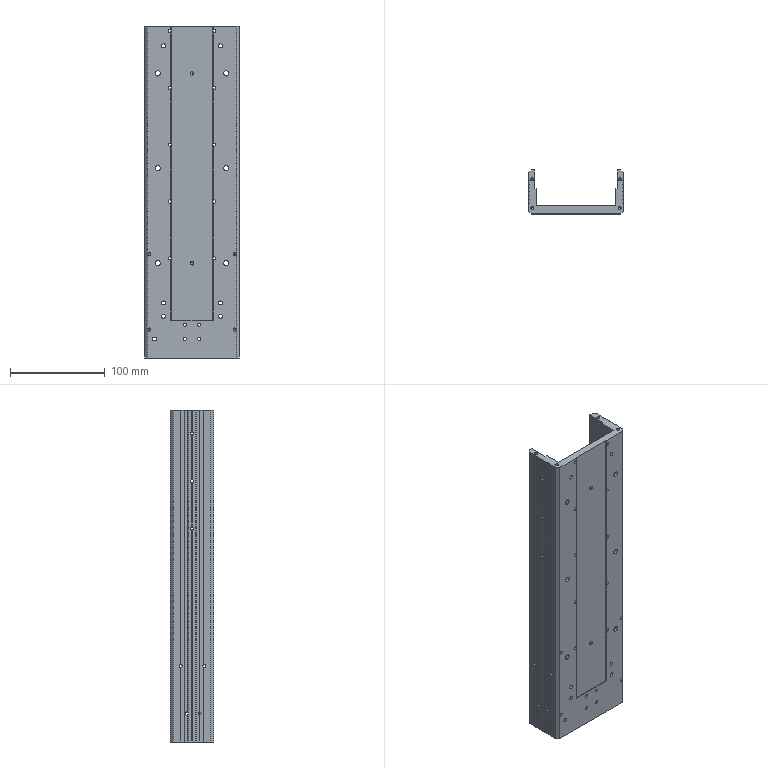Part | STEP file | lead screw 1.5Z module-direct connection | 1 solid | 290 faces | box 100 x 46 x 350 mm | volume 472702 mm3 | cylinder 136 | plane 122 | cone 32 | commonest cylinder face diameters 3.3 x90 4.2 x12 5.5 x12 9 x12 4 x6 10 x4